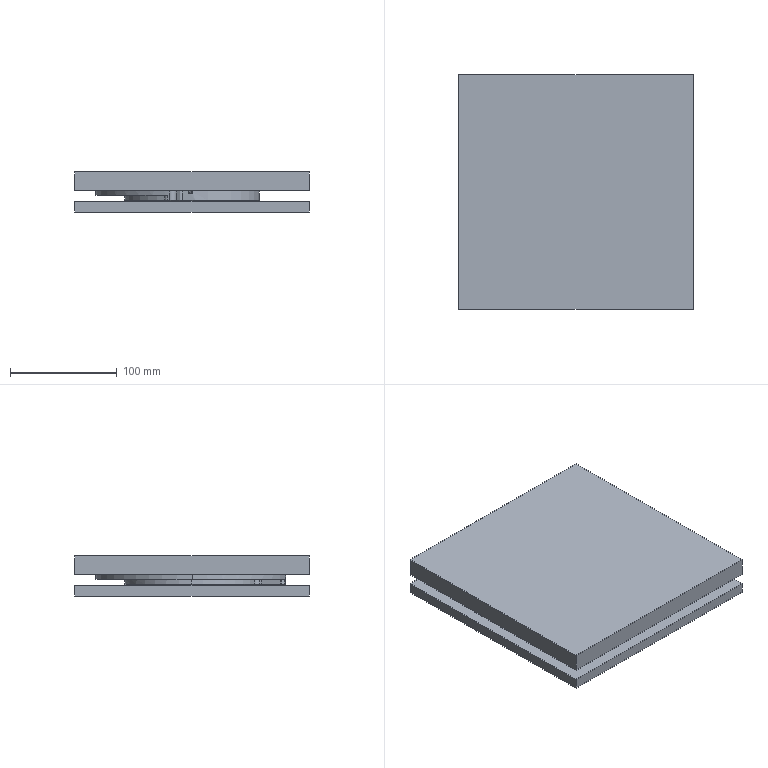NC program | NX | posted with a generic post | part box 220 x 220 x 37.5 mm
Lines 4727 to 4969 of 4969:
(FLOOR_WALL_COPY_COPY , TOOL : D10JING)
N9446 T07 M6
N9448 G54
N9450 G17 G0 G90 X-85.502 Y-44.552 S9500 M3
N9452 G43 Z30. H7
N9454 Z-11.
N9456 G94 G1 Z-12.5 F1000.
N9458 X-85.37 Y-44.454
N9460 G3 X-84.924 Y-42.578 R1.5
N9462 G2 X90.929 Y27.512 R-95.
N9464 G3 X81.541 Y30.681 R8.5
N9466 G1 X63.687 Y25.222
N9468 G3 X-56.664 Y-38.489 R-68.5
N9470 G1 X-70.985 Y-46.757
N9472 G2 X-84.924 Y-42.578 R10.
N9474 G1 X-79.56 Y-39.889
N9476 G2 X81.06 Y36.746 R-89.
N9478 G3 X79.787 Y36.419 R14.5
N9480 G1 X67.029 Y32.518
N9482 G3 X-65.013 Y-36.381 R-74.5
N9484 G1 X-73.985 Y-41.56
N9486 G2 X-79.56 Y-39.889 R4.
N9488 G1 X-75.124 Y-35.29
N9490 G2 X72.472 Y40.457 R83.
N9492 G1 X70.025 Y39.708
N9494 G3 X-72.951 Y-34.035 R80.5
N9496 G1 X-75.124 Y-35.29
N9498 G3 X-75.784 Y-37.102 R1.5
N9500 G1 Z-11.
N9502 G0 Z30.
N9504 X-55.334 Y-42.052
N9506 Z-11.
N9508 G1 Z-12.5
N9510 X-55.162 Y-41.874
N9512 G3 X-55.027 Y-39.95 R1.5
N9514 G2 X63.391 Y24.609 R-68.
N9516 G1 X81.687 Y30.203
N9518 G2 X91.634 Y25.027 R8.
N9520 G3 X93.269 Y24.005 R1.5
N9522 G1 X93.46 Y24.032
N9524 Z-11.
N9526 G0 Z30.
N9528 X-21.233 Y42.074
N9530 Z-16.
N9532 G1 Z-17.5
N9534 G3 X-21.401 Y40.153 R1.5
N9536 G1 X-25.442 Y45.924
N9538 G2 X39.614 Y34.452 R52.5
N9540 G1 X33.843 Y30.412
N9542 G3 X-21.401 Y40.153 R45.5
N9544 G1 X-20.998 Y41.633
N9546 G3 X-21.166 Y39.712 R1.5
N9548 G2 X33.766 Y29.747 R45.
N9550 G1 X40.354 Y34.36
N9552 G3 X-26.168 Y46.089 R53.
N9554 G1 X-21.555 Y39.501
N9556 G2 X-21.166 Y39.712 R45.
N9558 G3 X-20.445 Y41.5 R1.5
N9560 G1 X-20.519 Y41.728
N9562 Z-16.
N9564 G0 Z30.
N9566 M5
(DRILLING_COPY_1_COPY_2 , TOOL : D6A45)
N9568 T18 M6
N9570 G54
N9572 G17 G0 G90 X-28.146 Y-16.25 S3000 M3
N9574 G43 Z30. H18
N9576 G94 G81 G98 Z-1.55 F200. R3.
N9578 X0. Y32.5
N9580 X28.146 Y-16.25
N9582 G80
N9584 G0 X28.146 Y-16.25 Z30.
(DRILLING_COPY_1_COPY_2_COPY , TOOL : D6A45)
N9586 X26.5 Y0.
N9588 G81 Z-1.85 F200. R3.
N9590 X13.25 Y22.95
N9592 X-13.25
N9594 X-26.5 Y0.
N9596 X-13.25 Y-22.95
N9598 X13.25
N9600 G80
N9602 G0 X13.25 Y-22.95 Z30.
N9604 M5
(DRILLING_COPY_1_COPY_1_COPY_2 , TOOL : 2.6ZT)
N9606 T12 M6
N9608 G54
N9610 G17 G0 G90 X-28.146 Y-16.25 S3000 M3
N9612 G43 Z30. H12
N9614 G94 G83 G98 Z-6.751 F120. Q2. R3.
N9616 X28.146
N9618 X0. Y32.5
N9620 G80
N9622 G0 X0. Y32.5 Z30.
N9624 M5
(DRILLING_COPY_1_COPY_1_COPY_2_COPY , TOOL : 3.5ZT)
N9626 T17 M6
N9628 G54
N9630 G17 G0 G90 X26.5 Y0. S3000 M3
N9632 G43 Z30. H17
N9634 G94 G83 G98 Z-6.552 F120. Q2. R3.
N9636 X13.25 Y22.95
N9638 X-13.25
N9640 X-26.5 Y0.
N9642 X-13.25 Y-22.95
N9644 X13.25
N9646 G80
N9648 G0 X13.25 Y-22.95 Z30.
N9650 M5
(ZLEVEL_PROFILE_COPY_1_COPY_COPY_COPY_COPY_2_COPY_COPY_COPY , TOOL : D6A45)
N9652 T18 M6
N9654 G54
N9656 G17 G0 G90 X34.271 Y26.951 S7000 M3
N9658 G43 Z30. H18
N9660 Z-8.5
N9662 G94 G1 X35.486 Y26.384 F1000.
N9664 G3 X36.084 Y26.436 R0.6
N9666 G1 X42.672 Y31.049
N9668 G3 X43.431 Y36.98 R4.041
N9670 X-28.164 Y49.604 R57.041
N9672 X-29.479 Y43.771 R4.041
N9674 G1 X-24.866 Y37.183
N9676 G3 X-19.619 Y35.954 R4.041
N9678 G2 X30.733 Y27.075 R40.959
N9680 G3 X36.084 Y26.436 R4.041
N9682 X36.337 Y26.98 R0.6
N9684 G1 X36.247 Y28.015
N9686 G0 Z30.
N9688 X-34.753 Y40.482
N9690 Z-8.5
N9692 G1 X-35.48 Y41.741
N9694 G3 X-36. Y42.041 R0.6
N9696 X-39.541 Y38.5 R3.541
N9698 X-36. Y42.041 R-3.541
N9700 X-36.52 Y41.741 R0.6
N9702 G1 X-37.247 Y40.482
N9704 G0 Z30.
N9706 X52.318 Y-5.292
N9708 Z-8.5
N9710 G1 X53.228 Y-5.77
N9712 G3 X53.528 Y-5.25 R0.6
N9714 X52.237 Y-3.959 R1.291
N9716 X53.528 Y-5.25 R-1.291
N9718 X53.228 Y-4.73 R0.6
N9720 G1 X52.318 Y-5.208
N9722 G0 Z30.
N9724 X84.82 Y13.348
N9726 Z-8.5
N9728 G1 X84.207 Y14.078
N9730 G3 X83.643 Y14.283 R0.6
N9732 G1 X64.062 Y10.83
N9734 G3 X62.804 Y9.091 R1.541
N9736 G2 X59.157 Y22.965 R-63.459
N9738 G3 X64.719 Y20.266 R4.541
N9740 G1 X83.015 Y25.86
N9742 G2 X87.367 Y23.449 R3.459
N9744 X88.006 Y20.921 R90.459
N9746 X83.643 Y14.283 R5.459
N9748 G3 X83.184 Y13.897 R0.6
N9750 G1 X82.828 Y12.921
N9752 G0 Z30.
(ZLEVEL_PROFILE_COPY_1_COPY_COPY_COPY_COPY_2_COPY_COPY_COPY_COPY , TOOL : D6A45)
N9754 X-22.414 Y74.945
N9756 Z-13.5
N9758 G1 X-22.139 Y75.88
N9760 G3 X-22.659 Y76.18 R0.6
N9762 X-24.725 Y74.114 R2.066
N9764 X-22.659 Y76.18 R-2.066
N9766 X-23.178 Y75.88 R0.6
N9768 G1 X-22.903 Y74.945
N9770 G0 Z30.
N9772 X-76.345 Y17.678
N9774 Z-13.5
N9776 G1 X-77.28 Y17.953
N9778 G3 X-77.58 Y17.434 R0.6
N9780 X-75.514 Y15.367 R2.066
N9782 X-77.58 Y17.434 R-2.066
N9784 X-77.28 Y16.914 R0.6
N9786 G1 X-76.345 Y17.189
N9788 G0 Z30.
N9790 X35.429 Y69.884
N9792 Z-13.5
N9794 G1 X35.704 Y70.819
N9796 G3 X35.184 Y71.119 R0.6
N9798 X33.118 Y69.053 R2.066
N9800 X35.184 Y71.119 R-2.066
N9802 X34.665 Y70.819 R0.6
N9804 G1 X34.94 Y69.884
N9806 G0 Z30.
N9808 X-57.511 Y53.099
N9810 Z-13.5
N9812 G1 X-58.446 Y53.374
N9814 G3 X-58.746 Y52.855 R0.6
N9816 X-56.68 Y50.788 R2.066
N9818 X-58.746 Y52.855 R-2.066
N9820 X-58.446 Y52.335 R0.6
N9822 G1 X-57.511 Y52.61
N9824 G0 Z30.
N9826 X72.688 Y28.788
N9828 Z-13.5
N9830 G1 X73.623 Y28.512
N9832 G3 X73.923 Y29.032 R0.6
N9834 X71.857 Y31.098 R2.066
N9836 X73.923 Y29.032 R-2.066
N9838 X73.623 Y29.552 R0.6
N9840 G1 X72.688 Y29.277
N9842 G0 Z30.
N9844 X-74.945 Y-22.414
N9846 Z-13.5
N9848 G1 X-75.88 Y-22.139
N9850 G3 X-76.18 Y-22.659 R0.6
N9852 X-74.114 Y-24.725 R2.066
N9854 X-76.18 Y-22.659 R-2.066
N9856 X-75.88 Y-23.178 R0.6
N9858 G1 X-74.945 Y-22.903
N9860 G0 Z30.
N9862 X-57.001 Y-35.402
N9864 Z-13.5
N9866 G1 X-56.782 Y-33.936
N9868 X-56.836 Y-33.931
N9870 X-56.888 Y-33.945
N9872 X-56.932 Y-33.977
N9874 X-73.005 Y-43.257
N9876 G2 X-81.311 Y-40.767 R5.959
N9878 X86.416 Y28.385 R-90.959
N9880 G3 X86.863 Y27.984 R0.6
N9882 G1 X89.113 Y27.514
N9884 G0 Z30.
N9886 M5
N9888 M2